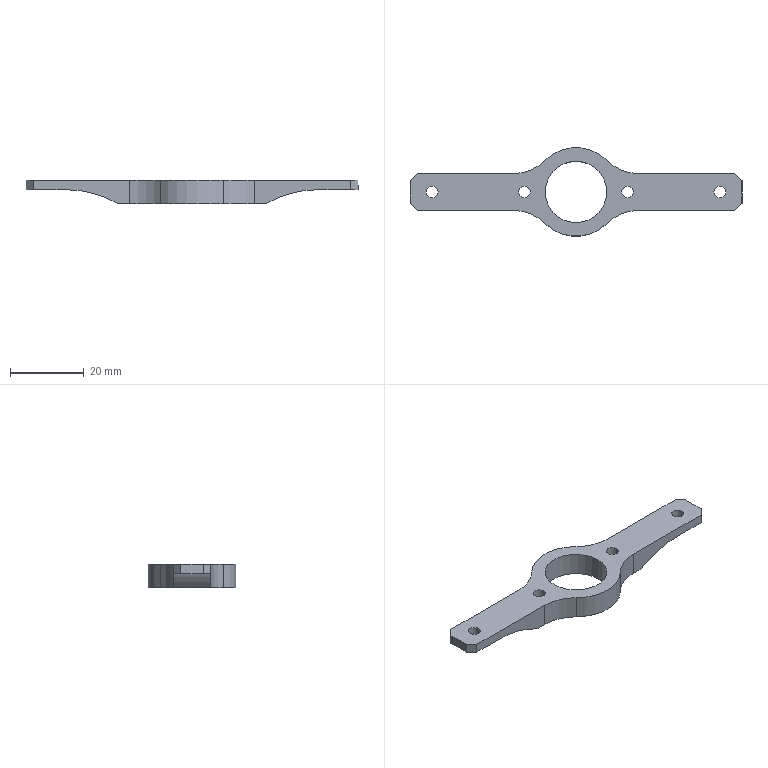Part | SolidWorks | features BaseBody 1 | 1 solid | 32 faces | box 90 x 24 x 6.35 mm | volume 4122 mm3 | cylinder 18 | plane 14 | commonest cylinder face diameters 3.2 x8 24 x6 16.667 x2 57.936 x2
STEP:
#1=CARTESIAN_POINT('',(46.666,0.,6.35));
#2=VERTEX_POINT('',#1);
#3=CARTESIAN_POINT('',(63.334,0.,6.35));
#4=VERTEX_POINT('',#3);
#5=CARTESIAN_POINT('',(55.,0.,6.35));
#6=DIRECTION('',(0.,0.,1.));
#7=DIRECTION('',(-1.,0.,0.));
#8=AXIS2_PLACEMENT_3D('',#5,#6,#7);
#9=CIRCLE('',#8,8.334);
#10=EDGE_CURVE('',#2,#4,#9,.T.);
#11=ORIENTED_EDGE('',*,*,#10,.T.);
#12=CARTESIAN_POINT('',(63.334,0.,0.));
#13=VERTEX_POINT('',#12);
#14=CARTESIAN_POINT('',(63.334,0.,6.35));
#15=DIRECTION('',(0.,0.,-1.));
#16=VECTOR('',#15,1000.);
#17=LINE('',#14,#16);
#18=EDGE_CURVE('',#4,#13,#17,.T.);
#19=ORIENTED_EDGE('',*,*,#18,.T.);
#20=CARTESIAN_POINT('',(46.666,0.,0.));
#21=VERTEX_POINT('',#20);
#22=CARTESIAN_POINT('',(55.,0.,0.));
#23=DIRECTION('',(0.,0.,-1.));
#24=DIRECTION('',(-1.,0.,0.));
#25=AXIS2_PLACEMENT_3D('',#22,#23,#24);
#26=CIRCLE('',#25,8.334);
#27=EDGE_CURVE('',#13,#21,#26,.T.);
#28=ORIENTED_EDGE('',*,*,#27,.T.);
#29=CARTESIAN_POINT('',(46.666,0.,6.35));
#30=DIRECTION('',(0.,0.,-1.));
#31=VECTOR('',#30,1000.);
#32=LINE('',#29,#31);
#33=EDGE_CURVE('',#2,#21,#32,.T.);
#34=ORIENTED_EDGE('',*,*,#33,.F.);
#35=EDGE_LOOP('',(#11,#19,#28,#34));
#36=FACE_OUTER_BOUND('',#35,.T.);
#37=CARTESIAN_POINT('',(55.,0.,6.35));
#38=DIRECTION('',(0.,0.,-1.));
#39=DIRECTION('',(-1.,0.,0.));
#40=AXIS2_PLACEMENT_3D('',#37,#38,#39);
#41=CYLINDRICAL_SURFACE('',#40,8.334);
#42=ADVANCED_FACE('',(#36),#41,.F.);
#43=CARTESIAN_POINT('',(67.4,0.,6.35));
#44=VERTEX_POINT('',#43);
#45=CARTESIAN_POINT('',(70.6,0.,6.35));
#46=VERTEX_POINT('',#45);
#47=CARTESIAN_POINT('',(69.,0.,6.35));
#48=DIRECTION('',(0.,0.,1.));
#49=DIRECTION('',(-1.,0.,0.));
#50=AXIS2_PLACEMENT_3D('',#47,#48,#49);
#51=CIRCLE('',#50,1.6);
#52=EDGE_CURVE('',#44,#46,#51,.T.);
#53=ORIENTED_EDGE('',*,*,#52,.T.);
#54=CARTESIAN_POINT('',(70.6,0.,0.));
#55=VERTEX_POINT('',#54);
#56=CARTESIAN_POINT('',(70.6,0.,6.35));
#57=DIRECTION('',(0.,0.,-1.));
#58=VECTOR('',#57,1000.);
#59=LINE('',#56,#58);
#60=EDGE_CURVE('',#46,#55,#59,.T.);
#61=ORIENTED_EDGE('',*,*,#60,.T.);
#62=CARTESIAN_POINT('',(67.4,0.,0.));
#63=VERTEX_POINT('',#62);
#64=CARTESIAN_POINT('',(69.,0.,0.));
#65=DIRECTION('',(0.,0.,1.));
#66=DIRECTION('',(-1.,0.,0.));
#67=AXIS2_PLACEMENT_3D('',#64,#65,#66);
#68=CIRCLE('',#67,1.6);
#69=EDGE_CURVE('',#63,#55,#68,.T.);
#70=ORIENTED_EDGE('',*,*,#69,.F.);
#71=CARTESIAN_POINT('',(67.4,0.,6.35));
#72=DIRECTION('',(0.,0.,-1.));
#73=VECTOR('',#72,1000.);
#74=LINE('',#71,#73);
#75=EDGE_CURVE('',#44,#63,#74,.T.);
#76=ORIENTED_EDGE('',*,*,#75,.F.);
#77=EDGE_LOOP('',(#53,#61,#70,#76));
#78=FACE_OUTER_BOUND('',#77,.T.);
#79=CARTESIAN_POINT('',(69.,0.,6.35));
#80=DIRECTION('',(0.,0.,-1.));
#81=DIRECTION('',(-1.,0.,0.));
#82=AXIS2_PLACEMENT_3D('',#79,#80,#81);
#83=CYLINDRICAL_SURFACE('',#82,1.6);
#84=ADVANCED_FACE('',(#78),#83,.F.);
#85=CARTESIAN_POINT('',(39.4,0.,6.35));
#86=VERTEX_POINT('',#85);
#87=CARTESIAN_POINT('',(42.6,0.,6.35));
#88=VERTEX_POINT('',#87);
#89=CARTESIAN_POINT('',(41.,0.,6.35));
#90=DIRECTION('',(0.,0.,1.));
#91=DIRECTION('',(-1.,0.,0.));
#92=AXIS2_PLACEMENT_3D('',#89,#90,#91);
#93=CIRCLE('',#92,1.6);
#94=EDGE_CURVE('',#86,#88,#93,.T.);
#95=ORIENTED_EDGE('',*,*,#94,.T.);
#96=CARTESIAN_POINT('',(42.6,0.,0.));
#97=VERTEX_POINT('',#96);
#98=CARTESIAN_POINT('',(42.6,0.,6.35));
#99=DIRECTION('',(0.,0.,-1.));
#100=VECTOR('',#99,1000.);
#101=LINE('',#98,#100);
#102=EDGE_CURVE('',#88,#97,#101,.T.);
#103=ORIENTED_EDGE('',*,*,#102,.T.);
#104=CARTESIAN_POINT('',(39.4,0.,0.));
#105=VERTEX_POINT('',#104);
#106=CARTESIAN_POINT('',(41.,0.,0.));
#107=DIRECTION('',(0.,0.,1.));
#108=DIRECTION('',(-1.,0.,0.));
#109=AXIS2_PLACEMENT_3D('',#106,#107,#108);
#110=CIRCLE('',#109,1.6);
#111=EDGE_CURVE('',#105,#97,#110,.T.);
#112=ORIENTED_EDGE('',*,*,#111,.F.);
#113=CARTESIAN_POINT('',(39.4,0.,6.35));
#114=DIRECTION('',(0.,0.,-1.));
#115=VECTOR('',#114,1000.);
#116=LINE('',#113,#115);
#117=EDGE_CURVE('',#86,#105,#116,.T.);
#118=ORIENTED_EDGE('',*,*,#117,.F.);
#119=EDGE_LOOP('',(#95,#103,#112,#118));
#120=FACE_OUTER_BOUND('',#119,.T.);
#121=CARTESIAN_POINT('',(41.,0.,6.35));
#122=DIRECTION('',(0.,0.,-1.));
#123=DIRECTION('',(-1.,0.,0.));
#124=AXIS2_PLACEMENT_3D('',#121,#122,#123);
#125=CYLINDRICAL_SURFACE('',#124,1.6);
#126=ADVANCED_FACE('',(#120),#125,.F.);
#127=CARTESIAN_POINT('',(14.4,0.,6.35));
#128=VERTEX_POINT('',#127);
#129=CARTESIAN_POINT('',(17.6,0.,6.35));
#130=VERTEX_POINT('',#129);
#131=CARTESIAN_POINT('',(16.,0.,6.35));
#132=DIRECTION('',(0.,0.,1.));
#133=DIRECTION('',(-1.,0.,0.));
#134=AXIS2_PLACEMENT_3D('',#131,#132,#133);
#135=CIRCLE('',#134,1.6);
#136=EDGE_CURVE('',#128,#130,#135,.T.);
#137=ORIENTED_EDGE('',*,*,#136,.T.);
#138=CARTESIAN_POINT('',(17.6,0.,3.81));
#139=VERTEX_POINT('',#138);
#140=CARTESIAN_POINT('',(17.6,0.,6.35));
#141=DIRECTION('',(0.,0.,-1.));
#142=VECTOR('',#141,1000.);
#143=LINE('',#140,#142);
#144=EDGE_CURVE('',#130,#139,#143,.T.);
#145=ORIENTED_EDGE('',*,*,#144,.T.);
#146=CARTESIAN_POINT('',(14.4,0.,3.81));
#147=VERTEX_POINT('',#146);
#148=CARTESIAN_POINT('',(16.,0.,3.81));
#149=DIRECTION('',(0.,0.,-1.));
#150=DIRECTION('',(-1.,0.,0.));
#151=AXIS2_PLACEMENT_3D('',#148,#149,#150);
#152=CIRCLE('',#151,1.6);
#153=EDGE_CURVE('',#139,#147,#152,.T.);
#154=ORIENTED_EDGE('',*,*,#153,.T.);
#155=CARTESIAN_POINT('',(14.4,0.,6.35));
#156=DIRECTION('',(0.,0.,-1.));
#157=VECTOR('',#156,1000.);
#158=LINE('',#155,#157);
#159=EDGE_CURVE('',#128,#147,#158,.T.);
#160=ORIENTED_EDGE('',*,*,#159,.F.);
#161=EDGE_LOOP('',(#137,#145,#154,#160));
#162=FACE_OUTER_BOUND('',#161,.T.);
#163=CARTESIAN_POINT('',(16.,0.,6.35));
#164=DIRECTION('',(0.,0.,-1.));
#165=DIRECTION('',(-1.,0.,0.));
#166=AXIS2_PLACEMENT_3D('',#163,#164,#165);
#167=CYLINDRICAL_SURFACE('',#166,1.6);
#168=ADVANCED_FACE('',(#162),#167,.F.);
#169=CARTESIAN_POINT('',(92.4,0.,6.35));
#170=VERTEX_POINT('',#169);
#171=CARTESIAN_POINT('',(95.6,0.,6.35));
#172=VERTEX_POINT('',#171);
#173=CARTESIAN_POINT('',(94.,0.,6.35));
#174=DIRECTION('',(0.,0.,1.));
#175=DIRECTION('',(-1.,0.,0.));
#176=AXIS2_PLACEMENT_3D('',#173,#174,#175);
#177=CIRCLE('',#176,1.6);
#178=EDGE_CURVE('',#170,#172,#177,.T.);
#179=ORIENTED_EDGE('',*,*,#178,.T.);
#180=CARTESIAN_POINT('',(95.6,0.,3.81));
#181=VERTEX_POINT('',#180);
#182=CARTESIAN_POINT('',(95.6,0.,6.35));
#183=DIRECTION('',(0.,0.,-1.));
#184=VECTOR('',#183,1000.);
#185=LINE('',#182,#184);
#186=EDGE_CURVE('',#172,#181,#185,.T.);
#187=ORIENTED_EDGE('',*,*,#186,.T.);
#188=CARTESIAN_POINT('',(92.4,0.,3.81));
#189=VERTEX_POINT('',#188);
#190=CARTESIAN_POINT('',(94.,0.,3.81));
#191=DIRECTION('',(0.,0.,-1.));
#192=DIRECTION('',(-1.,0.,0.));
#193=AXIS2_PLACEMENT_3D('',#190,#191,#192);
#194=CIRCLE('',#193,1.6);
#195=EDGE_CURVE('',#181,#189,#194,.T.);
#196=ORIENTED_EDGE('',*,*,#195,.T.);
#197=CARTESIAN_POINT('',(92.4,0.,6.35));
#198=DIRECTION('',(0.,0.,-1.));
#199=VECTOR('',#198,1000.);
#200=LINE('',#197,#199);
#201=EDGE_CURVE('',#170,#189,#200,.T.);
#202=ORIENTED_EDGE('',*,*,#201,.F.);
#203=EDGE_LOOP('',(#179,#187,#196,#202));
#204=FACE_OUTER_BOUND('',#203,.T.);
#205=CARTESIAN_POINT('',(94.,0.,6.35));
#206=DIRECTION('',(0.,0.,-1.));
#207=DIRECTION('',(-1.,0.,0.));
#208=AXIS2_PLACEMENT_3D('',#205,#206,#207);
#209=CYLINDRICAL_SURFACE('',#208,1.6);
#210=ADVANCED_FACE('',(#204),#209,.F.);
#211=ORIENTED_EDGE('',*,*,#18,.F.);
#212=CARTESIAN_POINT('',(55.,0.,6.35));
#213=DIRECTION('',(0.,0.,1.));
#214=DIRECTION('',(-1.,0.,0.));
#215=AXIS2_PLACEMENT_3D('',#212,#213,#214);
#216=CIRCLE('',#215,8.334);
#217=EDGE_CURVE('',#4,#2,#216,.T.);
#218=ORIENTED_EDGE('',*,*,#217,.T.);
#219=ORIENTED_EDGE('',*,*,#33,.T.);
#220=CARTESIAN_POINT('',(55.,0.,0.));
#221=DIRECTION('',(0.,0.,-1.));
#222=DIRECTION('',(-1.,0.,0.));
#223=AXIS2_PLACEMENT_3D('',#220,#221,#222);
#224=CIRCLE('',#223,8.334);
#225=EDGE_CURVE('',#21,#13,#224,.T.);
#226=ORIENTED_EDGE('',*,*,#225,.T.);
#227=EDGE_LOOP('',(#211,#218,#219,#226));
#228=FACE_OUTER_BOUND('',#227,.T.);
#229=CARTESIAN_POINT('',(55.,0.,6.35));
#230=DIRECTION('',(0.,0.,-1.));
#231=DIRECTION('',(-1.,0.,0.));
#232=AXIS2_PLACEMENT_3D('',#229,#230,#231);
#233=CYLINDRICAL_SURFACE('',#232,8.334);
#234=ADVANCED_FACE('',(#228),#233,.F.);
#235=ORIENTED_EDGE('',*,*,#225,.F.);
#236=ORIENTED_EDGE('',*,*,#27,.F.);
#237=EDGE_LOOP('',(#235,#236));
#238=FACE_BOUND('',#237,.T.);
#239=ORIENTED_EDGE('',*,*,#69,.T.);
#240=CARTESIAN_POINT('',(69.,0.,0.));
#241=DIRECTION('',(0.,0.,1.));
#242=DIRECTION('',(-1.,0.,0.));
#243=AXIS2_PLACEMENT_3D('',#240,#241,#242);
#244=CIRCLE('',#243,1.6);
#245=EDGE_CURVE('',#55,#63,#244,.T.);
#246=ORIENTED_EDGE('',*,*,#245,.T.);
#247=EDGE_LOOP('',(#239,#246));
#248=FACE_BOUND('',#247,.T.);
#249=ORIENTED_EDGE('',*,*,#111,.T.);
#250=CARTESIAN_POINT('',(41.,0.,0.));
#251=DIRECTION('',(0.,0.,1.));
#252=DIRECTION('',(-1.,0.,0.));
#253=AXIS2_PLACEMENT_3D('',#250,#251,#252);
#254=CIRCLE('',#253,1.6);
#255=EDGE_CURVE('',#97,#105,#254,.T.);
#256=ORIENTED_EDGE('',*,*,#255,.T.);
#257=EDGE_LOOP('',(#249,#256));
#258=FACE_BOUND('',#257,.T.);
#259=CARTESIAN_POINT('',(63.471,8.5,0.));
#260=VERTEX_POINT('',#259);
#261=CARTESIAN_POINT('',(71.941,5.,0.));
#262=VERTEX_POINT('',#261);
#263=CARTESIAN_POINT('',(71.941,17.,0.));
#264=DIRECTION('',(0.,0.,1.));
#265=DIRECTION('',(-1.,0.,0.));
#266=AXIS2_PLACEMENT_3D('',#263,#264,#265);
#267=CIRCLE('',#266,12.);
#268=EDGE_CURVE('',#260,#262,#267,.T.);
#269=ORIENTED_EDGE('',*,*,#268,.T.);
#270=CARTESIAN_POINT('',(75.,5.,0.));
#271=VERTEX_POINT('',#270);
#272=CARTESIAN_POINT('',(55.,5.,0.));
#273=DIRECTION('',(1.,0.,0.));
#274=VECTOR('',#273,1000.);
#275=LINE('',#272,#274);
#276=EDGE_CURVE('',#262,#271,#275,.T.);
#277=ORIENTED_EDGE('',*,*,#276,.T.);
#278=CARTESIAN_POINT('',(75.,-5.,0.));
#279=VERTEX_POINT('',#278);
#280=CARTESIAN_POINT('',(75.,0.,0.));
#281=DIRECTION('',(0.,-1.,0.));
#282=VECTOR('',#281,1000.);
#283=LINE('',#280,#282);
#284=EDGE_CURVE('',#271,#279,#283,.T.);
#285=ORIENTED_EDGE('',*,*,#284,.T.);
#286=CARTESIAN_POINT('',(71.941,-5.,0.));
#287=VERTEX_POINT('',#286);
#288=CARTESIAN_POINT('',(55.,-5.,0.));
#289=DIRECTION('',(-1.,0.,0.));
#290=VECTOR('',#289,1000.);
#291=LINE('',#288,#290);
#292=EDGE_CURVE('',#279,#287,#291,.T.);
#293=ORIENTED_EDGE('',*,*,#292,.T.);
#294=CARTESIAN_POINT('',(63.471,-8.5,0.));
#295=VERTEX_POINT('',#294);
#296=CARTESIAN_POINT('',(71.941,-17.,0.));
#297=DIRECTION('',(0.,0.,1.));
#298=DIRECTION('',(-1.,0.,0.));
#299=AXIS2_PLACEMENT_3D('',#296,#297,#298);
#300=CIRCLE('',#299,12.);
#301=EDGE_CURVE('',#287,#295,#300,.T.);
#302=ORIENTED_EDGE('',*,*,#301,.T.);
#303=CARTESIAN_POINT('',(46.529,-8.5,0.));
#304=VERTEX_POINT('',#303);
#305=CARTESIAN_POINT('',(55.,0.,0.));
#306=DIRECTION('',(0.,0.,-1.));
#307=DIRECTION('',(-1.,0.,0.));
#308=AXIS2_PLACEMENT_3D('',#305,#306,#307);
#309=CIRCLE('',#308,12.);
#310=EDGE_CURVE('',#295,#304,#309,.T.);
#311=ORIENTED_EDGE('',*,*,#310,.T.);
#312=CARTESIAN_POINT('',(38.059,-5.,0.));
#313=VERTEX_POINT('',#312);
#314=CARTESIAN_POINT('',(38.059,-17.,0.));
#315=DIRECTION('',(0.,0.,1.));
#316=DIRECTION('',(-1.,0.,0.));
#317=AXIS2_PLACEMENT_3D('',#314,#315,#316);
#318=CIRCLE('',#317,12.);
#319=EDGE_CURVE('',#304,#313,#318,.T.);
#320=ORIENTED_EDGE('',*,*,#319,.T.);
#321=CARTESIAN_POINT('',(35.,-5.,0.));
#322=VERTEX_POINT('',#321);
#323=CARTESIAN_POINT('',(55.,-5.,0.));
#324=DIRECTION('',(-1.,0.,0.));
#325=VECTOR('',#324,1000.);
#326=LINE('',#323,#325);
#327=EDGE_CURVE('',#313,#322,#326,.T.);
#328=ORIENTED_EDGE('',*,*,#327,.T.);
#329=CARTESIAN_POINT('',(35.,5.,0.));
#330=VERTEX_POINT('',#329);
#331=CARTESIAN_POINT('',(35.,0.,0.));
#332=DIRECTION('',(0.,1.,0.));
#333=VECTOR('',#332,1000.);
#334=LINE('',#331,#333);
#335=EDGE_CURVE('',#322,#330,#334,.T.);
#336=ORIENTED_EDGE('',*,*,#335,.T.);
#337=CARTESIAN_POINT('',(38.059,5.,0.));
#338=VERTEX_POINT('',#337);
#339=CARTESIAN_POINT('',(55.,5.,0.));
#340=DIRECTION('',(1.,0.,0.));
#341=VECTOR('',#340,1000.);
#342=LINE('',#339,#341);
#343=EDGE_CURVE('',#330,#338,#342,.T.);
#344=ORIENTED_EDGE('',*,*,#343,.T.);
#345=CARTESIAN_POINT('',(46.529,8.5,0.));
#346=VERTEX_POINT('',#345);
#347=CARTESIAN_POINT('',(38.059,17.,0.));
#348=DIRECTION('',(0.,0.,1.));
#349=DIRECTION('',(-1.,0.,0.));
#350=AXIS2_PLACEMENT_3D('',#347,#348,#349);
#351=CIRCLE('',#350,12.);
#352=EDGE_CURVE('',#338,#346,#351,.T.);
#353=ORIENTED_EDGE('',*,*,#352,.T.);
#354=CARTESIAN_POINT('',(55.,0.,0.));
#355=DIRECTION('',(0.,0.,-1.));
#356=DIRECTION('',(-1.,0.,0.));
#357=AXIS2_PLACEMENT_3D('',#354,#355,#356);
#358=CIRCLE('',#357,12.);
#359=EDGE_CURVE('',#346,#260,#358,.T.);
#360=ORIENTED_EDGE('',*,*,#359,.T.);
#361=EDGE_LOOP('',(#269,#277,#285,#293,#302,#311,#320,#328,#336,#344,#353,#360));
#362=FACE_OUTER_BOUND('',#361,.T.);
#363=CARTESIAN_POINT('',(75.,-12.144,0.));
#364=DIRECTION('',(0.,0.,-1.));
#365=DIRECTION('',(-1.,0.,0.));
#366=AXIS2_PLACEMENT_3D('',#363,#364,#365);
#367=PLANE('',#366);
#368=ADVANCED_FACE('',(#238,#248,#258,#362),#367,.T.);
#369=ORIENTED_EDGE('',*,*,#10,.F.);
#370=ORIENTED_EDGE('',*,*,#217,.F.);
#371=EDGE_LOOP('',(#369,#370));
#372=FACE_BOUND('',#371,.T.);
#373=ORIENTED_EDGE('',*,*,#136,.F.);
#374=CARTESIAN_POINT('',(16.,0.,6.35));
#375=DIRECTION('',(0.,0.,1.));
#376=DIRECTION('',(-1.,0.,0.));
#377=AXIS2_PLACEMENT_3D('',#374,#375,#376);
#378=CIRCLE('',#377,1.6);
#379=EDGE_CURVE('',#130,#128,#378,.T.);
#380=ORIENTED_EDGE('',*,*,#379,.F.);
#381=EDGE_LOOP('',(#373,#380));
#382=FACE_BOUND('',#381,.T.);
#383=ORIENTED_EDGE('',*,*,#94,.F.);
#384=CARTESIAN_POINT('',(41.,0.,6.35));
#385=DIRECTION('',(0.,0.,1.));
#386=DIRECTION('',(-1.,0.,0.));
#387=AXIS2_PLACEMENT_3D('',#384,#385,#386);
#388=CIRCLE('',#387,1.6);
#389=EDGE_CURVE('',#88,#86,#388,.T.);
#390=ORIENTED_EDGE('',*,*,#389,.F.);
#391=EDGE_LOOP('',(#383,#390));
#392=FACE_BOUND('',#391,.T.);
#393=ORIENTED_EDGE('',*,*,#178,.F.);
#394=CARTESIAN_POINT('',(94.,0.,6.35));
#395=DIRECTION('',(0.,0.,1.));
#396=DIRECTION('',(-1.,0.,0.));
#397=AXIS2_PLACEMENT_3D('',#394,#395,#396);
#398=CIRCLE('',#397,1.6);
#399=EDGE_CURVE('',#172,#170,#398,.T.);
#400=ORIENTED_EDGE('',*,*,#399,.F.);
#401=EDGE_LOOP('',(#393,#400));
#402=FACE_BOUND('',#401,.T.);
#403=ORIENTED_EDGE('',*,*,#52,.F.);
#404=CARTESIAN_POINT('',(69.,0.,6.35));
#405=DIRECTION('',(0.,0.,1.));
#406=DIRECTION('',(-1.,0.,0.));
#407=AXIS2_PLACEMENT_3D('',#404,#405,#406);
#408=CIRCLE('',#407,1.6);
#409=EDGE_CURVE('',#46,#44,#408,.T.);
#410=ORIENTED_EDGE('',*,*,#409,.F.);
#411=EDGE_LOOP('',(#403,#410));
#412=FACE_BOUND('',#411,.T.);
#413=CARTESIAN_POINT('',(12.,-5.,6.35));
#414=VERTEX_POINT('',#413);
#415=CARTESIAN_POINT('',(10.,-3.,6.35));
#416=VERTEX_POINT('',#415);
#417=CARTESIAN_POINT('',(12.,-5.,6.35));
#418=DIRECTION('',(-0.7071,0.7071,0.));
#419=VECTOR('',#418,1000.);
#420=LINE('',#417,#419);
#421=EDGE_CURVE('',#414,#416,#420,.T.);
#422=ORIENTED_EDGE('',*,*,#421,.F.);
#423=CARTESIAN_POINT('',(38.059,-5.,6.35));
#424=VERTEX_POINT('',#423);
#425=CARTESIAN_POINT('',(55.,-5.,6.35));
#426=DIRECTION('',(-1.,0.,0.));
#427=VECTOR('',#426,1000.);
#428=LINE('',#425,#427);
#429=EDGE_CURVE('',#424,#414,#428,.T.);
#430=ORIENTED_EDGE('',*,*,#429,.F.);
#431=CARTESIAN_POINT('',(46.529,-8.5,6.35));
#432=VERTEX_POINT('',#431);
#433=CARTESIAN_POINT('',(38.059,-17.,6.35));
#434=DIRECTION('',(0.,0.,1.));
#435=DIRECTION('',(-1.,0.,0.));
#436=AXIS2_PLACEMENT_3D('',#433,#434,#435);
#437=CIRCLE('',#436,12.);
#438=EDGE_CURVE('',#432,#424,#437,.T.);
#439=ORIENTED_EDGE('',*,*,#438,.F.);
#440=CARTESIAN_POINT('',(63.471,-8.5,6.35));
#441=VERTEX_POINT('',#440);
#442=CARTESIAN_POINT('',(55.,0.,6.35));
#443=DIRECTION('',(0.,0.,-1.));
#444=DIRECTION('',(-1.,0.,0.));
#445=AXIS2_PLACEMENT_3D('',#442,#443,#444);
#446=CIRCLE('',#445,12.);
#447=EDGE_CURVE('',#441,#432,#446,.T.);
#448=ORIENTED_EDGE('',*,*,#447,.F.);
#449=CARTESIAN_POINT('',(71.941,-5.,6.35));
#450=VERTEX_POINT('',#449);
#451=CARTESIAN_POINT('',(71.941,-17.,6.35));
#452=DIRECTION('',(0.,0.,1.));
#453=DIRECTION('',(-1.,0.,0.));
#454=AXIS2_PLACEMENT_3D('',#451,#452,#453);
#455=CIRCLE('',#454,12.);
#456=EDGE_CURVE('',#450,#441,#455,.T.);
#457=ORIENTED_EDGE('',*,*,#456,.F.);
#458=CARTESIAN_POINT('',(98.,-5.,6.35));
#459=VERTEX_POINT('',#458);
#460=CARTESIAN_POINT('',(55.,-5.,6.35));
#461=DIRECTION('',(-1.,0.,0.));
#462=VECTOR('',#461,1000.);
#463=LINE('',#460,#462);
#464=EDGE_CURVE('',#459,#450,#463,.T.);
#465=ORIENTED_EDGE('',*,*,#464,.F.);
#466=CARTESIAN_POINT('',(100.,-3.,6.35));
#467=VERTEX_POINT('',#466);
#468=CARTESIAN_POINT('',(100.,-3.,6.35));
#469=DIRECTION('',(-0.7071,-0.7071,0.));
#470=VECTOR('',#469,1000.);
#471=LINE('',#468,#470);
#472=EDGE_CURVE('',#467,#459,#471,.T.);
#473=ORIENTED_EDGE('',*,*,#472,.F.);
#474=CARTESIAN_POINT('',(100.,3.,6.35));
#475=VERTEX_POINT('',#474);
#476=CARTESIAN_POINT('',(100.,0.,6.35));
#477=DIRECTION('',(0.,-1.,0.));
#478=VECTOR('',#477,1000.);
#479=LINE('',#476,#478);
#480=EDGE_CURVE('',#475,#467,#479,.T.);
#481=ORIENTED_EDGE('',*,*,#480,.F.);
#482=CARTESIAN_POINT('',(98.,5.,6.35));
#483=VERTEX_POINT('',#482);
#484=CARTESIAN_POINT('',(98.,5.,6.35));
#485=DIRECTION('',(0.7071,-0.7071,0.));
#486=VECTOR('',#485,1000.);
#487=LINE('',#484,#486);
#488=EDGE_CURVE('',#483,#475,#487,.T.);
#489=ORIENTED_EDGE('',*,*,#488,.F.);
#490=CARTESIAN_POINT('',(71.941,5.,6.35));
#491=VERTEX_POINT('',#490);
#492=CARTESIAN_POINT('',(55.,5.,6.35));
#493=DIRECTION('',(1.,0.,0.));
#494=VECTOR('',#493,1000.);
#495=LINE('',#492,#494);
#496=EDGE_CURVE('',#491,#483,#495,.T.);
#497=ORIENTED_EDGE('',*,*,#496,.F.);
#498=CARTESIAN_POINT('',(63.471,8.5,6.35));
#499=VERTEX_POINT('',#498);
#500=CARTESIAN_POINT('',(71.941,17.,6.35));
#501=DIRECTION('',(0.,0.,1.));
#502=DIRECTION('',(-1.,0.,0.));
#503=AXIS2_PLACEMENT_3D('',#500,#501,#502);
#504=CIRCLE('',#503,12.);
#505=EDGE_CURVE('',#499,#491,#504,.T.);
#506=ORIENTED_EDGE('',*,*,#505,.F.);
#507=CARTESIAN_POINT('',(46.529,8.5,6.35));
#508=VERTEX_POINT('',#507);
#509=CARTESIAN_POINT('',(55.,0.,6.35));
#510=DIRECTION('',(0.,0.,-1.));
#511=DIRECTION('',(-1.,0.,0.));
#512=AXIS2_PLACEMENT_3D('',#509,#510,#511);
#513=CIRCLE('',#512,12.);
#514=EDGE_CURVE('',#508,#499,#513,.T.);
#515=ORIENTED_EDGE('',*,*,#514,.F.);
#516=CARTESIAN_POINT('',(38.059,5.,6.35));
#517=VERTEX_POINT('',#516);
#518=CARTESIAN_POINT('',(38.059,17.,6.35));
#519=DIRECTION('',(0.,0.,1.));
#520=DIRECTION('',(-1.,0.,0.));
#521=AXIS2_PLACEMENT_3D('',#518,#519,#520);
#522=CIRCLE('',#521,12.);
#523=EDGE_CURVE('',#517,#508,#522,.T.);
#524=ORIENTED_EDGE('',*,*,#523,.F.);
#525=CARTESIAN_POINT('',(12.,5.,6.35));
#526=VERTEX_POINT('',#525);
#527=CARTESIAN_POINT('',(55.,5.,6.35));
#528=DIRECTION('',(1.,0.,0.));
#529=VECTOR('',#528,1000.);
#530=LINE('',#527,#529);
#531=EDGE_CURVE('',#526,#517,#530,.T.);
#532=ORIENTED_EDGE('',*,*,#531,.F.);
#533=CARTESIAN_POINT('',(10.,3.,6.35));
#534=VERTEX_POINT('',#533);
#535=CARTESIAN_POINT('',(10.,3.,6.35));
#536=DIRECTION('',(0.7071,0.7071,0.));
#537=VECTOR('',#536,1000.);
#538=LINE('',#535,#537);
#539=EDGE_CURVE('',#534,#526,#538,.T.);
#540=ORIENTED_EDGE('',*,*,#539,.F.);
#541=CARTESIAN_POINT('',(10.,0.,6.35));
#542=DIRECTION('',(0.,1.,0.));
#543=VECTOR('',#542,1000.);
#544=LINE('',#541,#543);
#545=EDGE_CURVE('',#416,#534,#544,.T.);
#546=ORIENTED_EDGE('',*,*,#545,.F.);
#547=EDGE_LOOP('',(#422,#430,#439,#448,#457,#465,#473,#481,#489,#497,#506,#515,#524,#532,#540,#546));
#548=FACE_OUTER_BOUND('',#547,.T.);
#549=CARTESIAN_POINT('',(100.,-12.144,6.35));
#550=DIRECTION('',(0.,0.,-1.));
#551=DIRECTION('',(-1.,0.,0.));
#552=AXIS2_PLACEMENT_3D('',#549,#550,#551);
#553=PLANE('',#552);
#554=ADVANCED_FACE('',(#372,#382,#392,#402,#412,#548),#553,.F.);
#555=ORIENTED_EDGE('',*,*,#60,.F.);
#556=ORIENTED_EDGE('',*,*,#409,.T.);
#557=ORIENTED_EDGE('',*,*,#75,.T.);
#558=ORIENTED_EDGE('',*,*,#245,.F.);
#559=EDGE_LOOP('',(#555,#556,#557,#558));
#560=FACE_OUTER_BOUND('',#559,.T.);
#561=CARTESIAN_POINT('',(69.,0.,6.35));
#562=DIRECTION('',(0.,0.,-1.));
#563=DIRECTION('',(-1.,0.,0.));
#564=AXIS2_PLACEMENT_3D('',#561,#562,#563);
#565=CYLINDRICAL_SURFACE('',#564,1.6);
#566=ADVANCED_FACE('',(#560),#565,.F.);
#567=ORIENTED_EDGE('',*,*,#102,.F.);
#568=ORIENTED_EDGE('',*,*,#389,.T.);
#569=ORIENTED_EDGE('',*,*,#117,.T.);
#570=ORIENTED_EDGE('',*,*,#255,.F.);
#571=EDGE_LOOP('',(#567,#568,#569,#570));
#572=FACE_OUTER_BOUND('',#571,.T.);
#573=CARTESIAN_POINT('',(41.,0.,6.35));
#574=DIRECTION('',(0.,0.,-1.));
#575=DIRECTION('',(-1.,0.,0.));
#576=AXIS2_PLACEMENT_3D('',#573,#574,#575);
#577=CYLINDRICAL_SURFACE('',#576,1.6);
#578=ADVANCED_FACE('',(#572),#577,.F.);
#579=CARTESIAN_POINT('',(89.36,5.,3.81));
#580=VERTEX_POINT('',#579);
#581=CARTESIAN_POINT('',(98.,5.,3.81));
#582=VERTEX_POINT('',#581);
#583=CARTESIAN_POINT('',(84.971,5.,3.81));
#584=DIRECTION('',(1.,0.,0.));
#585=VECTOR('',#584,1000.);
#586=LINE('',#583,#585);
#587=EDGE_CURVE('',#580,#582,#586,.T.);
#588=ORIENTED_EDGE('',*,*,#587,.F.);
#589=CARTESIAN_POINT('',(89.36,5.,-25.158));
#590=DIRECTION('',(0.,1.,0.));
#591=DIRECTION('',(-1.,0.,0.));
#592=AXIS2_PLACEMENT_3D('',#589,#590,#591);
#593=CIRCLE('',#592,28.968);
#594=EDGE_CURVE('',#271,#580,#593,.T.);
#595=ORIENTED_EDGE('',*,*,#594,.F.);
#596=ORIENTED_EDGE('',*,*,#276,.F.);
#597=CARTESIAN_POINT('',(71.941,5.,3.175));
#598=DIRECTION('',(0.,0.,-1.));
#599=VECTOR('',#598,1000.);
#600=LINE('',#597,#599);
#601=EDGE_CURVE('',#491,#262,#600,.T.);
#602=ORIENTED_EDGE('',*,*,#601,.F.);
#603=ORIENTED_EDGE('',*,*,#496,.T.);
#604=CARTESIAN_POINT('',(98.,5.,3.175));
#605=DIRECTION('',(0.,0.,1.));
#606=VECTOR('',#605,1000.);
#607=LINE('',#604,#606);
#608=EDGE_CURVE('',#582,#483,#607,.T.);
#609=ORIENTED_EDGE('',*,*,#608,.F.);
#610=EDGE_LOOP('',(#588,#595,#596,#602,#603,#609));
#611=FACE_OUTER_BOUND('',#610,.T.);
#612=CARTESIAN_POINT('',(71.941,5.,0.));
#613=DIRECTION('',(0.,-1.,0.));
#614=DIRECTION('',(1.,0.,0.));
#615=AXIS2_PLACEMENT_3D('',#612,#613,#614);
#616=PLANE('',#615);
#617=ADVANCED_FACE('',(#611),#616,.F.);
#618=ORIENTED_EDGE('',*,*,#505,.T.);
#619=ORIENTED_EDGE('',*,*,#601,.T.);
#620=ORIENTED_EDGE('',*,*,#268,.F.);
#621=CARTESIAN_POINT('',(63.471,8.5,3.175));
#622=DIRECTION('',(0.,0.,1.));
#623=VECTOR('',#622,1000.);
#624=LINE('',#621,#623);
#625=EDGE_CURVE('',#260,#499,#624,.T.);
#626=ORIENTED_EDGE('',*,*,#625,.T.);
#627=EDGE_LOOP('',(#618,#619,#620,#626));
#628=FACE_OUTER_BOUND('',#627,.T.);
#629=CARTESIAN_POINT('',(71.941,17.,6.35));
#630=DIRECTION('',(0.,0.,-1.));
#631=DIRECTION('',(-1.,0.,0.));
#632=AXIS2_PLACEMENT_3D('',#629,#630,#631);
#633=CYLINDRICAL_SURFACE('',#632,12.);
#634=ADVANCED_FACE('',(#628),#633,.F.);
#635=CARTESIAN_POINT('',(46.529,8.5,3.175));
#636=DIRECTION('',(0.,0.,-1.));
#637=VECTOR('',#636,1000.);
#638=LINE('',#635,#637);
#639=EDGE_CURVE('',#508,#346,#638,.T.);
#640=ORIENTED_EDGE('',*,*,#639,.F.);
#641=ORIENTED_EDGE('',*,*,#514,.T.);
#642=ORIENTED_EDGE('',*,*,#625,.F.);
#643=ORIENTED_EDGE('',*,*,#359,.F.);
#644=EDGE_LOOP('',(#640,#641,#642,#643));
#645=FACE_OUTER_BOUND('',#644,.T.);
#646=CARTESIAN_POINT('',(55.,0.,6.35));
#647=DIRECTION('',(0.,0.,-1.));
#648=DIRECTION('',(-1.,0.,0.));
#649=AXIS2_PLACEMENT_3D('',#646,#647,#648);
#650=CYLINDRICAL_SURFACE('',#649,12.);
#651=ADVANCED_FACE('',(#645),#650,.T.);
#652=ORIENTED_EDGE('',*,*,#523,.T.);
#653=ORIENTED_EDGE('',*,*,#639,.T.);
#654=ORIENTED_EDGE('',*,*,#352,.F.);
#655=CARTESIAN_POINT('',(38.059,5.,3.175));
#656=DIRECTION('',(0.,0.,1.));
#657=VECTOR('',#656,1000.);
#658=LINE('',#655,#657);
#659=EDGE_CURVE('',#338,#517,#658,.T.);
#660=ORIENTED_EDGE('',*,*,#659,.T.);
#661=EDGE_LOOP('',(#652,#653,#654,#660));
#662=FACE_OUTER_BOUND('',#661,.T.);
#663=CARTESIAN_POINT('',(38.059,17.,6.35));
#664=DIRECTION('',(0.,0.,-1.));
#665=DIRECTION('',(-1.,0.,0.));
#666=AXIS2_PLACEMENT_3D('',#663,#664,#665);
#667=CYLINDRICAL_SURFACE('',#666,12.);
#668=ADVANCED_FACE('',(#662),#667,.F.);
#669=CARTESIAN_POINT('',(12.,5.,3.81));
#670=VERTEX_POINT('',#669);
#671=CARTESIAN_POINT('',(12.,5.,3.175));
#672=DIRECTION('',(0.,0.,-1.));
#673=VECTOR('',#672,1000.);
#674=LINE('',#671,#673);
#675=EDGE_CURVE('',#526,#670,#674,.T.);
#676=ORIENTED_EDGE('',*,*,#675,.F.);
#677=ORIENTED_EDGE('',*,*,#531,.T.);
#678=ORIENTED_EDGE('',*,*,#659,.F.);
#679=ORIENTED_EDGE('',*,*,#343,.F.);
#680=CARTESIAN_POINT('',(20.64,5.,3.81));
#681=VERTEX_POINT('',#680);
#682=CARTESIAN_POINT('',(20.64,5.,-25.158));
#683=DIRECTION('',(0.,1.,0.));
#684=DIRECTION('',(-1.,0.,0.));
#685=AXIS2_PLACEMENT_3D('',#682,#683,#684);
#686=CIRCLE('',#685,28.968);
#687=EDGE_CURVE('',#681,#330,#686,.T.);
#688=ORIENTED_EDGE('',*,*,#687,.F.);
#689=CARTESIAN_POINT('',(25.029,5.,3.81));
#690=DIRECTION('',(1.,0.,0.));
#691=VECTOR('',#690,1000.);
#692=LINE('',#689,#691);
#693=EDGE_CURVE('',#670,#681,#692,.T.);
#694=ORIENTED_EDGE('',*,*,#693,.F.);
#695=EDGE_LOOP('',(#676,#677,#678,#679,#688,#694));
#696=FACE_OUTER_BOUND('',#695,.T.);
#697=CARTESIAN_POINT('',(12.,5.,0.));
#698=DIRECTION('',(0.,-1.,0.));
#699=DIRECTION('',(1.,0.,0.));
#700=AXIS2_PLACEMENT_3D('',#697,#698,#699);
#701=PLANE('',#700);
#702=ADVANCED_FACE('',(#696),#701,.F.);
#703=CARTESIAN_POINT('',(20.64,-5.,3.81));
#704=VERTEX_POINT('',#703);
#705=CARTESIAN_POINT('',(20.64,0.,3.81));
#706=DIRECTION('',(0.,1.,0.));
#707=VECTOR('',#706,1000.);
#708=LINE('',#705,#707);
#709=EDGE_CURVE('',#704,#681,#708,.T.);
#710=ORIENTED_EDGE('',*,*,#709,.T.);
#711=ORIENTED_EDGE('',*,*,#687,.T.);
#712=ORIENTED_EDGE('',*,*,#335,.F.);
#713=CARTESIAN_POINT('',(20.64,-5.,-25.158));
#714=DIRECTION('',(0.,-1.,0.));
#715=DIRECTION('',(-1.,0.,0.));
#716=AXIS2_PLACEMENT_3D('',#713,#714,#715);
#717=CIRCLE('',#716,28.968);
#718=EDGE_CURVE('',#322,#704,#717,.T.);
#719=ORIENTED_EDGE('',*,*,#718,.T.);
#720=EDGE_LOOP('',(#710,#711,#712,#719));
#721=FACE_OUTER_BOUND('',#720,.T.);
#722=CARTESIAN_POINT('',(20.64,-5.,-25.158));
#723=DIRECTION('',(0.,1.,0.));
#724=DIRECTION('',(-1.,0.,0.));
#725=AXIS2_PLACEMENT_3D('',#722,#723,#724);
#726=CYLINDRICAL_SURFACE('',#725,28.968);
#727=ADVANCED_FACE('',(#721),#726,.F.);
#728=CARTESIAN_POINT('',(12.,-5.,3.81));
#729=VERTEX_POINT('',#728);
#730=CARTESIAN_POINT('',(12.,-5.,3.175));
#731=DIRECTION('',(0.,0.,1.));
#732=VECTOR('',#731,1000.);
#733=LINE('',#730,#732);
#734=EDGE_CURVE('',#729,#414,#733,.T.);
#735=ORIENTED_EDGE('',*,*,#734,.F.);
#736=CARTESIAN_POINT('',(25.029,-5.,3.81));
#737=DIRECTION('',(-1.,0.,0.));
#738=VECTOR('',#737,1000.);
#739=LINE('',#736,#738);
#740=EDGE_CURVE('',#704,#729,#739,.T.);
#741=ORIENTED_EDGE('',*,*,#740,.F.);
#742=ORIENTED_EDGE('',*,*,#718,.F.);
#743=ORIENTED_EDGE('',*,*,#327,.F.);
#744=CARTESIAN_POINT('',(38.059,-5.,3.175));
#745=DIRECTION('',(0.,0.,-1.));
#746=VECTOR('',#745,1000.);
#747=LINE('',#744,#746);
#748=EDGE_CURVE('',#424,#313,#747,.T.);
#749=ORIENTED_EDGE('',*,*,#748,.F.);
#750=ORIENTED_EDGE('',*,*,#429,.T.);
#751=EDGE_LOOP('',(#735,#741,#742,#743,#749,#750));
#752=FACE_OUTER_BOUND('',#751,.T.);
#753=CARTESIAN_POINT('',(38.059,-5.,0.));
#754=DIRECTION('',(0.,1.,0.));
#755=DIRECTION('',(-1.,0.,0.));
#756=AXIS2_PLACEMENT_3D('',#753,#754,#755);
#757=PLANE('',#756);
#758=ADVANCED_FACE('',(#752),#757,.F.);
#759=ORIENTED_EDGE('',*,*,#438,.T.);
#760=ORIENTED_EDGE('',*,*,#748,.T.);
#761=ORIENTED_EDGE('',*,*,#319,.F.);
#762=CARTESIAN_POINT('',(46.529,-8.5,3.175));
#763=DIRECTION('',(0.,0.,1.));
#764=VECTOR('',#763,1000.);
#765=LINE('',#762,#764);
#766=EDGE_CURVE('',#304,#432,#765,.T.);
#767=ORIENTED_EDGE('',*,*,#766,.T.);
#768=EDGE_LOOP('',(#759,#760,#761,#767));
#769=FACE_OUTER_BOUND('',#768,.T.);
#770=CARTESIAN_POINT('',(38.059,-17.,6.35));
#771=DIRECTION('',(0.,0.,-1.));
#772=DIRECTION('',(-1.,0.,0.));
#773=AXIS2_PLACEMENT_3D('',#770,#771,#772);
#774=CYLINDRICAL_SURFACE('',#773,12.);
#775=ADVANCED_FACE('',(#769),#774,.F.);
#776=CARTESIAN_POINT('',(63.471,-8.5,3.175));
#777=DIRECTION('',(0.,0.,-1.));
#778=VECTOR('',#777,1000.);
#779=LINE('',#776,#778);
#780=EDGE_CURVE('',#441,#295,#779,.T.);
#781=ORIENTED_EDGE('',*,*,#780,.F.);
#782=ORIENTED_EDGE('',*,*,#447,.T.);
#783=ORIENTED_EDGE('',*,*,#766,.F.);
#784=ORIENTED_EDGE('',*,*,#310,.F.);
#785=EDGE_LOOP('',(#781,#782,#783,#784));
#786=FACE_OUTER_BOUND('',#785,.T.);
#787=CARTESIAN_POINT('',(55.,0.,6.35));
#788=DIRECTION('',(0.,0.,-1.));
#789=DIRECTION('',(-1.,0.,0.));
#790=AXIS2_PLACEMENT_3D('',#787,#788,#789);
#791=CYLINDRICAL_SURFACE('',#790,12.);
#792=ADVANCED_FACE('',(#786),#791,.T.);
#793=ORIENTED_EDGE('',*,*,#456,.T.);
#794=ORIENTED_EDGE('',*,*,#780,.T.);
#795=ORIENTED_EDGE('',*,*,#301,.F.);
#796=CARTESIAN_POINT('',(71.941,-5.,3.175));
#797=DIRECTION('',(0.,0.,1.));
#798=VECTOR('',#797,1000.);
#799=LINE('',#796,#798);
#800=EDGE_CURVE('',#287,#450,#799,.T.);
#801=ORIENTED_EDGE('',*,*,#800,.T.);
#802=EDGE_LOOP('',(#793,#794,#795,#801));
#803=FACE_OUTER_BOUND('',#802,.T.);
#804=CARTESIAN_POINT('',(71.941,-17.,6.35));
#805=DIRECTION('',(0.,0.,-1.));
#806=DIRECTION('',(-1.,0.,0.));
#807=AXIS2_PLACEMENT_3D('',#804,#805,#806);
#808=CYLINDRICAL_SURFACE('',#807,12.);
#809=ADVANCED_FACE('',(#803),#808,.F.);
#810=CARTESIAN_POINT('',(98.,-5.,3.81));
#811=VERTEX_POINT('',#810);
#812=CARTESIAN_POINT('',(89.36,-5.,3.81));
#813=VERTEX_POINT('',#812);
#814=CARTESIAN_POINT('',(84.971,-5.,3.81));
#815=DIRECTION('',(-1.,0.,0.));
#816=VECTOR('',#815,1000.);
#817=LINE('',#814,#816);
#818=EDGE_CURVE('',#811,#813,#817,.T.);
#819=ORIENTED_EDGE('',*,*,#818,.F.);
#820=CARTESIAN_POINT('',(98.,-5.,3.175));
#821=DIRECTION('',(0.,0.,-1.));
#822=VECTOR('',#821,1000.);
#823=LINE('',#820,#822);
#824=EDGE_CURVE('',#459,#811,#823,.T.);
#825=ORIENTED_EDGE('',*,*,#824,.F.);
#826=ORIENTED_EDGE('',*,*,#464,.T.);
#827=ORIENTED_EDGE('',*,*,#800,.F.);
#828=ORIENTED_EDGE('',*,*,#292,.F.);
#829=CARTESIAN_POINT('',(89.36,-5.,-25.158));
#830=DIRECTION('',(0.,-1.,0.));
#831=DIRECTION('',(-1.,0.,0.));
#832=AXIS2_PLACEMENT_3D('',#829,#830,#831);
#833=CIRCLE('',#832,28.968);
#834=EDGE_CURVE('',#813,#279,#833,.T.);
#835=ORIENTED_EDGE('',*,*,#834,.F.);
#836=EDGE_LOOP('',(#819,#825,#826,#827,#828,#835));
#837=FACE_OUTER_BOUND('',#836,.T.);
#838=CARTESIAN_POINT('',(98.,-5.,0.));
#839=DIRECTION('',(0.,1.,0.));
#840=DIRECTION('',(-1.,0.,0.));
#841=AXIS2_PLACEMENT_3D('',#838,#839,#840);
#842=PLANE('',#841);
#843=ADVANCED_FACE('',(#837),#842,.F.);
#844=CARTESIAN_POINT('',(89.36,0.,3.81));
#845=DIRECTION('',(0.,-1.,0.));
#846=VECTOR('',#845,1000.);
#847=LINE('',#844,#846);
#848=EDGE_CURVE('',#580,#813,#847,.T.);
#849=ORIENTED_EDGE('',*,*,#848,.T.);
#850=ORIENTED_EDGE('',*,*,#834,.T.);
#851=ORIENTED_EDGE('',*,*,#284,.F.);
#852=ORIENTED_EDGE('',*,*,#594,.T.);
#853=EDGE_LOOP('',(#849,#850,#851,#852));
#854=FACE_OUTER_BOUND('',#853,.T.);
#855=CARTESIAN_POINT('',(89.36,-5.,-25.158));
#856=DIRECTION('',(0.,1.,0.));
#857=DIRECTION('',(-1.,0.,0.));
#858=AXIS2_PLACEMENT_3D('',#855,#856,#857);
#859=CYLINDRICAL_SURFACE('',#858,28.968);
#860=ADVANCED_FACE('',(#854),#859,.F.);
#861=ORIENTED_EDGE('',*,*,#144,.F.);
#862=ORIENTED_EDGE('',*,*,#379,.T.);
#863=ORIENTED_EDGE('',*,*,#159,.T.);
#864=CARTESIAN_POINT('',(16.,0.,3.81));
#865=DIRECTION('',(0.,0.,-1.));
#866=DIRECTION('',(-1.,0.,0.));
#867=AXIS2_PLACEMENT_3D('',#864,#865,#866);
#868=CIRCLE('',#867,1.6);
#869=EDGE_CURVE('',#147,#139,#868,.T.);
#870=ORIENTED_EDGE('',*,*,#869,.T.);
#871=EDGE_LOOP('',(#861,#862,#863,#870));
#872=FACE_OUTER_BOUND('',#871,.T.);
#873=CARTESIAN_POINT('',(16.,0.,6.35));
#874=DIRECTION('',(0.,0.,-1.));
#875=DIRECTION('',(-1.,0.,0.));
#876=AXIS2_PLACEMENT_3D('',#873,#874,#875);
#877=CYLINDRICAL_SURFACE('',#876,1.6);
#878=ADVANCED_FACE('',(#872),#877,.F.);
#879=ORIENTED_EDGE('',*,*,#186,.F.);
#880=ORIENTED_EDGE('',*,*,#399,.T.);
#881=ORIENTED_EDGE('',*,*,#201,.T.);
#882=CARTESIAN_POINT('',(94.,0.,3.81));
#883=DIRECTION('',(0.,0.,-1.));
#884=DIRECTION('',(-1.,0.,0.));
#885=AXIS2_PLACEMENT_3D('',#882,#883,#884);
#886=CIRCLE('',#885,1.6);
#887=EDGE_CURVE('',#189,#181,#886,.T.);
#888=ORIENTED_EDGE('',*,*,#887,.T.);
#889=EDGE_LOOP('',(#879,#880,#881,#888));
#890=FACE_OUTER_BOUND('',#889,.T.);
#891=CARTESIAN_POINT('',(94.,0.,6.35));
#892=DIRECTION('',(0.,0.,-1.));
#893=DIRECTION('',(-1.,0.,0.));
#894=AXIS2_PLACEMENT_3D('',#891,#892,#893);
#895=CYLINDRICAL_SURFACE('',#894,1.6);
#896=ADVANCED_FACE('',(#890),#895,.F.);
#897=CARTESIAN_POINT('',(10.,-3.,3.81));
#898=VERTEX_POINT('',#897);
#899=CARTESIAN_POINT('',(10.,3.,3.81));
#900=VERTEX_POINT('',#899);
#901=CARTESIAN_POINT('',(10.,0.,3.81));
#902=DIRECTION('',(0.,1.,0.));
#903=VECTOR('',#902,1000.);
#904=LINE('',#901,#903);
#905=EDGE_CURVE('',#898,#900,#904,.T.);
#906=ORIENTED_EDGE('',*,*,#905,.F.);
#907=CARTESIAN_POINT('',(10.,-3.,5.08));
#908=DIRECTION('',(0.,0.,-1.));
#909=VECTOR('',#908,1000.);
#910=LINE('',#907,#909);
#911=EDGE_CURVE('',#416,#898,#910,.T.);
#912=ORIENTED_EDGE('',*,*,#911,.F.);
#913=ORIENTED_EDGE('',*,*,#545,.T.);
#914=CARTESIAN_POINT('',(10.,3.,5.08));
#915=DIRECTION('',(0.,0.,1.));
#916=VECTOR('',#915,1000.);
#917=LINE('',#914,#916);
#918=EDGE_CURVE('',#900,#534,#917,.T.);
#919=ORIENTED_EDGE('',*,*,#918,.F.);
#920=EDGE_LOOP('',(#906,#912,#913,#919));
#921=FACE_OUTER_BOUND('',#920,.T.);
#922=CARTESIAN_POINT('',(10.,-3.,6.35));
#923=DIRECTION('',(1.,0.,0.));
#924=DIRECTION('',(0.,0.,-1.));
#925=AXIS2_PLACEMENT_3D('',#922,#923,#924);
#926=PLANE('',#925);
#927=ADVANCED_FACE('',(#921),#926,.F.);
#928=CARTESIAN_POINT('',(11.,-4.,3.81));
#929=DIRECTION('',(-0.7071,0.7071,0.));
#930=VECTOR('',#929,1000.);
#931=LINE('',#928,#930);
#932=EDGE_CURVE('',#729,#898,#931,.T.);
#933=ORIENTED_EDGE('',*,*,#932,.F.);
#934=ORIENTED_EDGE('',*,*,#734,.T.);
#935=ORIENTED_EDGE('',*,*,#421,.T.);
#936=ORIENTED_EDGE('',*,*,#911,.T.);
#937=EDGE_LOOP('',(#933,#934,#935,#936));
#938=FACE_OUTER_BOUND('',#937,.T.);
#939=CARTESIAN_POINT('',(12.,-5.,3.81));
#940=DIRECTION('',(0.7071,0.7071,0.));
#941=DIRECTION('',(-0.7071,0.7071,0.));
#942=AXIS2_PLACEMENT_3D('',#939,#940,#941);
#943=PLANE('',#942);
#944=ADVANCED_FACE('',(#938),#943,.F.);
#945=CARTESIAN_POINT('',(100.,-3.,3.81));
#946=VERTEX_POINT('',#945);
#947=CARTESIAN_POINT('',(99.,-4.,3.81));
#948=DIRECTION('',(-0.7071,-0.7071,0.));
#949=VECTOR('',#948,1000.);
#950=LINE('',#947,#949);
#951=EDGE_CURVE('',#946,#811,#950,.T.);
#952=ORIENTED_EDGE('',*,*,#951,.F.);
#953=CARTESIAN_POINT('',(100.,-3.,5.08));
#954=DIRECTION('',(0.,0.,-1.));
#955=VECTOR('',#954,1000.);
#956=LINE('',#953,#955);
#957=EDGE_CURVE('',#467,#946,#956,.T.);
#958=ORIENTED_EDGE('',*,*,#957,.F.);
#959=ORIENTED_EDGE('',*,*,#472,.T.);
#960=ORIENTED_EDGE('',*,*,#824,.T.);
#961=EDGE_LOOP('',(#952,#958,#959,#960));
#962=FACE_OUTER_BOUND('',#961,.T.);
#963=CARTESIAN_POINT('',(100.,-3.,3.81));
#964=DIRECTION('',(-0.7071,0.7071,0.));
#965=DIRECTION('',(-0.7071,-0.7071,0.));
#966=AXIS2_PLACEMENT_3D('',#963,#964,#965);
#967=PLANE('',#966);
#968=ADVANCED_FACE('',(#962),#967,.F.);
#969=CARTESIAN_POINT('',(100.,3.,3.81));
#970=VERTEX_POINT('',#969);
#971=CARTESIAN_POINT('',(100.,0.,3.81));
#972=DIRECTION('',(0.,-1.,0.));
#973=VECTOR('',#972,1000.);
#974=LINE('',#971,#973);
#975=EDGE_CURVE('',#970,#946,#974,.T.);
#976=ORIENTED_EDGE('',*,*,#975,.F.);
#977=CARTESIAN_POINT('',(100.,3.,5.08));
#978=DIRECTION('',(0.,0.,-1.));
#979=VECTOR('',#978,1000.);
#980=LINE('',#977,#979);
#981=EDGE_CURVE('',#475,#970,#980,.T.);
#982=ORIENTED_EDGE('',*,*,#981,.F.);
#983=ORIENTED_EDGE('',*,*,#480,.T.);
#984=ORIENTED_EDGE('',*,*,#957,.T.);
#985=EDGE_LOOP('',(#976,#982,#983,#984));
#986=FACE_OUTER_BOUND('',#985,.T.);
#987=CARTESIAN_POINT('',(100.,-3.,3.81));
#988=DIRECTION('',(-1.,0.,0.));
#989=DIRECTION('',(0.,0.,1.));
#990=AXIS2_PLACEMENT_3D('',#987,#988,#989);
#991=PLANE('',#990);
#992=ADVANCED_FACE('',(#986),#991,.F.);
#993=CARTESIAN_POINT('',(99.,4.,3.81));
#994=DIRECTION('',(0.7071,-0.7071,0.));
#995=VECTOR('',#994,1000.);
#996=LINE('',#993,#995);
#997=EDGE_CURVE('',#582,#970,#996,.T.);
#998=ORIENTED_EDGE('',*,*,#997,.F.);
#999=ORIENTED_EDGE('',*,*,#608,.T.);
#1000=ORIENTED_EDGE('',*,*,#488,.T.);
#1001=ORIENTED_EDGE('',*,*,#981,.T.);
#1002=EDGE_LOOP('',(#998,#999,#1000,#1001));
#1003=FACE_OUTER_BOUND('',#1002,.T.);
#1004=CARTESIAN_POINT('',(98.,5.,3.81));
#1005=DIRECTION('',(-0.7071,-0.7071,0.));
#1006=DIRECTION('',(0.7071,-0.7071,0.));
#1007=AXIS2_PLACEMENT_3D('',#1004,#1005,#1006);
#1008=PLANE('',#1007);
#1009=ADVANCED_FACE('',(#1003),#1008,.F.);
#1010=CARTESIAN_POINT('',(11.,4.,3.81));
#1011=DIRECTION('',(0.7071,0.7071,0.));
#1012=VECTOR('',#1011,1000.);
#1013=LINE('',#1010,#1012);
#1014=EDGE_CURVE('',#900,#670,#1013,.T.);
#1015=ORIENTED_EDGE('',*,*,#1014,.F.);
#1016=ORIENTED_EDGE('',*,*,#918,.T.);
#1017=ORIENTED_EDGE('',*,*,#539,.T.);
#1018=ORIENTED_EDGE('',*,*,#675,.T.);
#1019=EDGE_LOOP('',(#1015,#1016,#1017,#1018));
#1020=FACE_OUTER_BOUND('',#1019,.T.);
#1021=CARTESIAN_POINT('',(10.,3.,3.81));
#1022=DIRECTION('',(0.7071,-0.7071,0.));
#1023=DIRECTION('',(0.7071,0.7071,0.));
#1024=AXIS2_PLACEMENT_3D('',#1021,#1022,#1023);
#1025=PLANE('',#1024);
#1026=ADVANCED_FACE('',(#1020),#1025,.F.);
#1027=ORIENTED_EDGE('',*,*,#887,.F.);
#1028=ORIENTED_EDGE('',*,*,#195,.F.);
#1029=EDGE_LOOP('',(#1027,#1028));
#1030=FACE_BOUND('',#1029,.T.);
#1031=ORIENTED_EDGE('',*,*,#587,.T.);
#1032=ORIENTED_EDGE('',*,*,#997,.T.);
#1033=ORIENTED_EDGE('',*,*,#975,.T.);
#1034=ORIENTED_EDGE('',*,*,#951,.T.);
#1035=ORIENTED_EDGE('',*,*,#818,.T.);
#1036=ORIENTED_EDGE('',*,*,#848,.F.);
#1037=EDGE_LOOP('',(#1031,#1032,#1033,#1034,#1035,#1036));
#1038=FACE_OUTER_BOUND('',#1037,.T.);
#1039=CARTESIAN_POINT('',(89.36,-5.,3.81));
#1040=DIRECTION('',(0.,0.,1.));
#1041=DIRECTION('',(1.,0.,0.));
#1042=AXIS2_PLACEMENT_3D('',#1039,#1040,#1041);
#1043=PLANE('',#1042);
#1044=ADVANCED_FACE('',(#1030,#1038),#1043,.F.);
#1045=ORIENTED_EDGE('',*,*,#869,.F.);
#1046=ORIENTED_EDGE('',*,*,#153,.F.);
#1047=EDGE_LOOP('',(#1045,#1046));
#1048=FACE_BOUND('',#1047,.T.);
#1049=ORIENTED_EDGE('',*,*,#932,.T.);
#1050=ORIENTED_EDGE('',*,*,#905,.T.);
#1051=ORIENTED_EDGE('',*,*,#1014,.T.);
#1052=ORIENTED_EDGE('',*,*,#693,.T.);
#1053=ORIENTED_EDGE('',*,*,#709,.F.);
#1054=ORIENTED_EDGE('',*,*,#740,.T.);
#1055=EDGE_LOOP('',(#1049,#1050,#1051,#1052,#1053,#1054));
#1056=FACE_OUTER_BOUND('',#1055,.T.);
#1057=CARTESIAN_POINT('',(10.,-5.,3.81));
#1058=DIRECTION('',(0.,0.,1.));
#1059=DIRECTION('',(1.,0.,0.));
#1060=AXIS2_PLACEMENT_3D('',#1057,#1058,#1059);
#1061=PLANE('',#1060);
#1062=ADVANCED_FACE('',(#1048,#1056),#1061,.F.);
#1063=CLOSED_SHELL('',(#42,#84,#126,#168,#210,#234,#368,#554,#566,#578,#617,#634,#651,#668,#702,#727,#758,#775,#792,#809,#843,#860,#878,#896,#927,#944,#968,#992,#1009,#1026,#1044,#1062));
#1064=MANIFOLD_SOLID_BREP('',#1063);
#1065=CARTESIAN_POINT('',(0.,0.,0.));
#1066=DIRECTION('',(0.,0.,1.));
#1067=DIRECTION('',(1.,0.,0.));
#1068=AXIS2_PLACEMENT_3D('',#1065,#1066,#1067);
#1069=(LENGTH_UNIT()NAMED_UNIT(*)SI_UNIT(.MILLI.,.METRE.));
#1070=UNCERTAINTY_MEASURE_WITH_UNIT(LENGTH_MEASURE(0.00001),#1069,'','');
#1071=(NAMED_UNIT(*)PLANE_ANGLE_UNIT()SI_UNIT($,.RADIAN.));
#1072=(NAMED_UNIT(*)SI_UNIT($,.STERADIAN.)SOLID_ANGLE_UNIT());
#1073=(GEOMETRIC_REPRESENTATION_CONTEXT(3)GLOBAL_UNCERTAINTY_ASSIGNED_CONTEXT((#1070))GLOBAL_UNIT_ASSIGNED_CONTEXT((#1069,#1071,#1072))REPRESENTATION_CONTEXT('',''));
#1074=ADVANCED_BREP_SHAPE_REPRESENTATION('',(#1064,#1068),#1073);